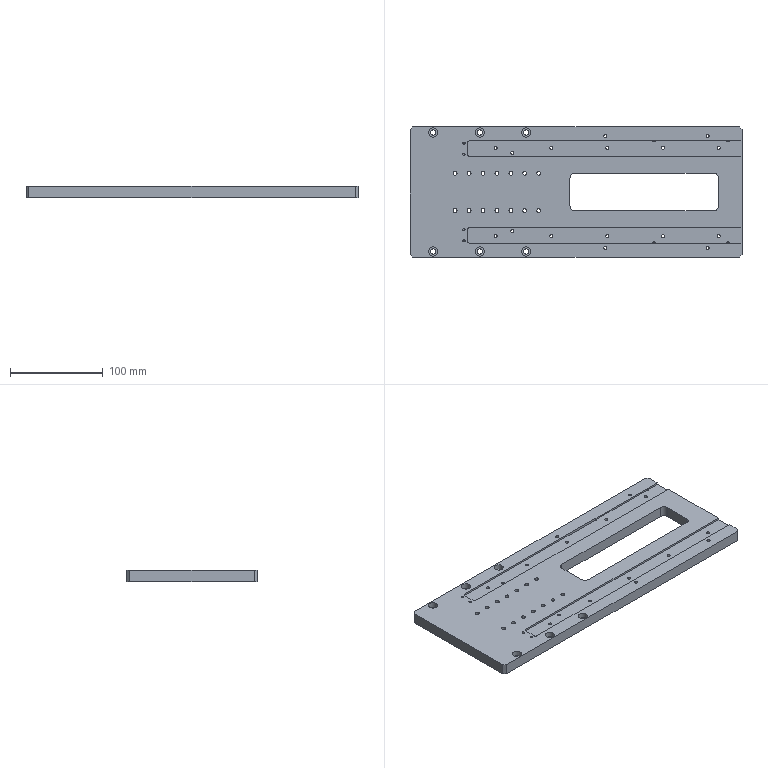NC program | NX | posted with a generic post | part box 357 x 140 x 12 mm
Whole program:
N10 G17 G21 G94 G90
(DRILLING , TOOL : D6A45)
N12 T01 M6
N14 G54
N16 G17 G0 G90 X153.5 Y-47.5 B0. C0. S9500 M3
N18 G43 Z30. H1
N20 G94 G81 G98 Z-1. F250. R3.
N22 X141.5 Y-60.
N24 X93.5 Y-47.5
N26 X33.5
N28 X31.5 Y-60.
N30 X-26.5 Y-47.5
N32 X-53.5 Y-64.
N34 X-68.5 Y-42.
N36 X-86.5 Y-47.5
N38 X-103.5 Y-64.
N40 X-120.5 Y-52.5
N42 X-153.5 Y-64.
N44 X-120.5 Y-40.5
N46 X-130. Y-20.
N48 X-115.
N50 X-100.
N52 X-85.
N54 X-70.
N56 X-55.
N58 X-40.
N60 Y20.
N62 X-55.
N64 X-70.
N66 X-85.
N68 X-100.
N70 X-115.
N72 X-130.
N74 X-120.5 Y40.5
N76 X-153.5 Y64.
N78 X-120.5 Y52.5
N80 X-103.5 Y64.
N82 X-86.5 Y47.5
N84 X-68.5 Y42.
N86 X-53.5 Y64.
N88 X-26.5 Y47.5
N90 X31.5 Y60.
N92 X33.5 Y47.5
N94 X93.5
N96 X141.5 Y60.
N98 X153.5 Y47.5
N100 G80
N102 G0 X153.5 Y47.5 Z30.
N104 M5
(DRILLING_COPY_COPY_COPY , TOOL : 2.5ZT)
N106 T02 M6
N108 G54
N110 G17 G0 G90 X-120.5 Y52.5 B0. C0. S2000 M3
N112 G43 Z30. H2
N114 G94 G83 G98 Z-8.101 F100. Q2. R3.
N116 Y40.5
N118 Y-40.5
N120 Y-52.5
N122 G80
N124 G0 X-120.5 Y-52.5 Z30.
N126 M5
(DRILLING_COPY_COPY , TOOL : 5.5ZT)
N128 T09 M6
N130 G54
N132 G17 G0 G90 X-153.5 Y-64. B0. C0. S2000 M3
N134 G43 Z30. H9
N136 G94 G83 G98 Z-14.152 F300. Q2. R3.
N138 X-103.5
N140 X-53.5
N142 Y64.
N144 X-103.5
N146 X-153.5
N148 G80
N150 G0 X-153.5 Y64. Z30.
N152 M5
(DRILLING_COPY_COPY_COPY_COPY , TOOL : 4.2ZT)
N154 T04 M6
N156 G54
N158 G17 G0 G90 X-40. Y20. B0. C0. S2000 M3
N160 G43 Z30. H4
N162 G94 G83 G98 Z-13.762 F300. Q2. R3.
N164 X-55.
N166 X-70.
N168 X-85.
N170 X-100.
N172 X-115.
N174 X-130.
N176 Y-20.
N178 X-115.
N180 X-100.
N182 X-85.
N184 X-70.
N186 X-55.
N188 X-40.
N190 G80
N192 G0 X-40. Y-20. Z30.
N194 M5
(DRILLING_COPY_COPY_COPY_1 , TOOL : 3.3ZT)
N196 T03 M6
N198 G54
N200 G17 G0 G90 X-86.5 Y-47.5 B0. C0. S2026 M3
N202 G43 Z30. H3
N204 G94 G83 G98 Z-13.491 F200. Q2. R3.
N206 X-68.5 Y-42.
N208 X-26.5 Y-47.5
N210 X33.5
N212 X93.5
N214 X153.5
N216 Y47.5
N218 X93.5
N220 X33.5
N222 X-26.5
N224 X-68.5 Y42.
N226 X-86.5 Y47.5
N228 G80
N230 G0 X-86.5 Y47.5 Z30.
N232 M5
(ZLEVEL_PROFILE , TOOL : D10)
N234 T15 M6
N236 G54
N238 G17 G0 G90 X175.718 Y79.678 B0. C0. S9500 M3
N240 G43 Z30. H15
N242 Z0.5
N244 G94 G1 Z-1. F1000.
N246 X175.3 Y78.117
N248 G3 X175.558 Y77.151 R1.
N250 G1 X178.707 Y74.002 F3000.
N252 X179.106 Y73.606
N254 X182.106 Y70.606
N256 G2 X183.6 Y67. R5.1
N258 G1 Y-65.997
N260 X183.537 Y-66.201
N262 G2 X182.106 Y-70.606 R5.1
N264 G1 X180.619 Y-72.094
N266 X180.58 Y-72.128
N268 X175.558 Y-77.151
N270 G3 X175.3 Y-78.117 R1.
N272 G1 X175.72 Y-79.686
N274 Z0.5
N276 G0 Z-0.5
N278 G1 Z-2. F1000.
N280 X175.3 Y-78.117
N282 G2 X175.558 Y-77.151 R1.
N284 G1 X180.58 Y-72.128 F3000.
N286 X182.106 Y-70.606
N288 G3 X183.537 Y-66.201 R5.1
N290 G1 X183.6 Y-65.997
N292 Y67.
N294 G3 X182.106 Y70.606 R5.1
N296 G1 X179.106 Y73.606
N298 X178.707 Y74.002
N300 X175.558 Y77.151
N302 G2 X175.3 Y78.117 R1.
N304 G1 X175.718 Y79.678
N306 Z-0.5
N308 G0 Z-1.5
N310 G1 Z-3. F1000.
N312 X175.3 Y78.117
N314 G3 X175.558 Y77.151 R1.
N316 G1 X178.707 Y74.002 F3000.
N318 X179.106 Y73.606
N320 X182.106 Y70.606
N322 G2 X183.6 Y67. R5.1
N324 G1 Y-65.997
N326 X183.537 Y-66.201
N328 G2 X182.106 Y-70.606 R5.1
N330 G1 X180.581 Y-72.128
N332 X175.558 Y-77.151
N334 G3 X175.3 Y-78.117 R1.
N336 G1 X175.72 Y-79.686
N338 Z-1.5
N340 G0 Z-2.5
N342 G1 Z-4. F1000.
N344 X175.3 Y-78.117
N346 G2 X175.559 Y-77.152 R1.
N348 G1 X180.619 Y-72.094 F3000.
N350 X182.106 Y-70.606
N352 G3 X183.537 Y-66.201 R5.1
N354 G1 X183.6 Y-65.997
N356 Y67.
N358 G3 X182.106 Y70.606 R5.1
N360 G1 X179.106 Y73.606
N362 X178.707 Y74.002
N364 X175.559 Y77.152
N366 G2 X175.3 Y78.117 R1.
N368 G1 X175.718 Y79.678
N370 Z-2.5
N372 G0 Z-3.5
N374 G1 Z-5. F1000.
N376 X175.3 Y78.118
N378 G3 X175.559 Y77.152 R1.
N380 G1 X178.707 Y74.002 F3000.
N382 X179.106 Y73.606
N384 X182.106 Y70.606
N386 G2 X183.6 Y67. R5.1
N388 G1 Y-65.997
N390 X183.537 Y-66.201
N392 G2 X182.106 Y-70.606 R5.1
N394 G1 X180.581 Y-72.128
N396 X175.559 Y-77.152
N398 G3 X175.3 Y-78.118 R1.
N400 G1 X175.721 Y-79.687
N402 Z-3.5
N404 G0 Z-4.5
N406 G1 Z-6. F1000.
N408 X175.3 Y-78.118
N410 G2 X175.559 Y-77.152 R1.
N412 G1 X180.619 Y-72.094 F3000.
N414 X182.106 Y-70.606
N416 G3 X183.537 Y-66.201 R5.1
N418 G1 X183.6 Y-65.997
N420 Y67.
N422 G3 X182.106 Y70.606 R5.1
N424 G1 X179.106 Y73.606
N426 X175.559 Y77.152
N428 G2 X175.3 Y78.118 R1.
N430 G1 X175.718 Y79.679
N432 Z-4.5
N434 G0 Z-5.5
N436 G1 Z-7. F1000.
N438 X175.3 Y78.118
N440 G3 X175.559 Y77.152 R1.
N442 G1 X179.106 Y73.606 F3000.
N444 X182.106 Y70.606
N446 G2 X183.6 Y67. R5.1
N448 G1 Y-65.997
N450 X183.537 Y-66.201
N452 G2 X182.106 Y-70.606 R5.1
N454 G1 X180.581 Y-72.128
N456 X175.559 Y-77.152
N458 G3 X175.3 Y-78.118 R1.
N460 G1 X175.721 Y-79.687
N462 Z-5.5
N464 G0 Z-6.5
N466 G1 Z-8. F1000.
N468 X175.3 Y-78.118
N470 G2 X175.559 Y-77.152 R1.
N472 G1 X180.619 Y-72.094 F3000.
N474 X182.106 Y-70.606
N476 G3 X183.537 Y-66.201 R5.1
N478 G1 X183.6 Y-65.997
N480 Y67.
N482 G3 X182.106 Y70.606 R5.1
N484 G1 X179.106 Y73.606
N486 X175.559 Y77.152
N488 G2 X175.3 Y78.118 R1.
N490 G1 X175.718 Y79.679
N492 Z-6.5
N494 G0 Z-7.5
N496 G1 Z-9. F1000.
N498 X175.3 Y78.118
N500 G3 X175.559 Y77.152 R1.
N502 G1 X179.106 Y73.606 F3000.
N504 X182.106 Y70.606
N506 G2 X183.6 Y67. R5.1
N508 G1 Y-65.997
N510 X183.537 Y-66.201
N512 G2 X182.106 Y-70.606 R5.1
N514 G1 X180.619 Y-72.094
N516 X175.559 Y-77.152
N518 G3 X175.3 Y-78.118 R1.
N520 G1 X175.72 Y-79.687
N522 Z-7.5
N524 G0 Z-8.5
N526 G1 Z-10. F1000.
N528 X175.3 Y-78.118
N530 G2 X175.559 Y-77.152 R1.
N532 G1 X180.619 Y-72.094 F3000.
N534 X182.106 Y-70.606
N536 G3 X183.537 Y-66.201 R5.1
N538 G1 X183.6 Y-65.997
N540 Y67.
N542 G3 X182.106 Y70.606 R5.1
N544 G1 X179.106 Y73.606
N546 X175.559 Y77.152
N548 G2 X175.3 Y78.118 R1.
N550 G1 X175.718 Y79.679
N552 Z-8.5
N554 G0 Z-9.5
N556 G1 Z-11. F1000.
N558 X175.3 Y78.118
N560 G3 X175.559 Y77.152 R1.
N562 G1 X179.106 Y73.606 F3000.
N564 X182.106 Y70.606
N566 G2 X183.6 Y67. R5.1
N568 G1 Y-65.997
N570 X183.537 Y-66.201
N572 G2 X182.106 Y-70.606 R5.1
N574 G1 X180.619 Y-72.094
N576 X175.559 Y-77.152
N578 G3 X175.3 Y-78.118 R1.
N580 G1 X175.721 Y-79.687
N582 Z-9.5
N584 G0 Y-79.688 Z-10.5
N586 G1 Z-12. F1000.
N588 X175.3 Y-78.118
N590 G2 X175.559 Y-77.152 R1.
N592 G1 X180.619 Y-72.094 F3000.
N594 X182.106 Y-70.606
N596 G3 X183.537 Y-66.201 R5.1
N598 G1 X183.6 Y-65.997
N600 Y67.
N602 G3 X182.106 Y70.606 R5.1
N604 G1 X179.106 Y73.606
N606 X175.559 Y77.152
N608 G2 X175.3 Y78.118 R1.
N610 G1 X175.718 Y79.679
N612 Z-10.5
N614 G0 Z30.
N616 X-175.718 Y-79.678
N618 Z0.5
N620 G1 Z-1. F1000.
N622 X-175.3 Y-78.117
N624 G3 X-175.558 Y-77.151 R1.
N626 G1 X-180.58 Y-72.128 F3000.
N628 X-180.619 Y-72.094
N630 X-182.106 Y-70.606
N632 G2 X-183.569 Y-66.438 R5.1
N634 G1 X-183.596 Y-66.387
N636 Y-65.997
N638 X-183.6 Y-65.948
N640 Y67.
N642 G2 X-182.106 Y70.606 R5.1
N644 G1 X-179.106 Y73.606
N646 X-178.51 Y74.198
N648 X-175.558 Y77.151
N650 G3 X-175.3 Y78.117 R1.
N652 G1 X-175.72 Y79.686
N654 Z0.5
N656 G0 Z-0.5
N658 G1 Z-2. F1000.
N660 X-175.3 Y78.117
N662 G2 X-175.558 Y77.151 R1.
N664 G1 X-178.51 Y74.198 F3000.
N666 X-179.106 Y73.606
N668 X-182.106 Y70.606
N670 G3 X-183.6 Y67. R5.1
N672 G1 Y-65.948
N674 X-183.596 Y-65.997
N676 Y-66.387
N678 X-183.569 Y-66.438
N680 G3 X-182.106 Y-70.606 R5.1
N682 G1 X-180.58 Y-72.128
N684 X-175.558 Y-77.151
N686 G2 X-175.3 Y-78.117 R1.
N688 G1 X-175.718 Y-79.678
N690 Z-0.5
N692 G0 Z-1.5
N694 G1 Z-3. F1000.
N696 X-175.3 Y-78.117
N698 G3 X-175.558 Y-77.151 R1.
N700 G1 X-180.619 Y-72.094 F3000.
N702 X-182.106 Y-70.606
N704 G2 X-183.569 Y-66.438 R5.1
N706 G1 X-183.596 Y-66.387
N708 Y-65.997
N710 X-183.6 Y-65.948
N712 Y67.
N714 G2 X-182.106 Y70.606 R5.1
N716 G1 X-179.106 Y73.606
N718 X-178.51 Y74.198
N720 X-175.558 Y77.151
N722 G3 X-175.3 Y78.117 R1.
N724 G1 X-175.721 Y79.686
N726 Z-1.5
N728 G0 Z-2.5
N730 G1 Z-4. F1000.
N732 X-175.3 Y78.117
N734 G2 X-175.559 Y77.152 R1.
N736 G1 X-178.511 Y74.198 F3000.
N738 X-179.106 Y73.606
N740 X-182.106 Y70.606
N742 G3 X-183.6 Y67. R5.1
N744 G1 Y-65.948
N746 X-183.596 Y-65.997
N748 Y-66.387
N750 X-183.569 Y-66.438
N752 G3 X-182.106 Y-70.606 R5.1
N754 G1 X-180.581 Y-72.128
N756 X-175.559 Y-77.152
N758 G2 X-175.3 Y-78.117 R1.
N760 G1 X-175.718 Y-79.678
N762 Z-2.5
N764 G0 Z-3.5
N766 G1 Z-5. F1000.
N768 X-175.3 Y-78.118
N770 G3 X-175.559 Y-77.152 R1.
N772 G1 X-180.619 Y-72.094 F3000.
N774 X-182.106 Y-70.606
N776 G2 X-183.569 Y-66.438 R5.1
N778 G1 X-183.596 Y-66.387
N780 Y-65.997
N782 X-183.6 Y-65.948
N784 Y67.
N786 G2 X-182.106 Y70.606 R5.1
N788 G1 X-179.106 Y73.606
N790 X-178.511 Y74.199
N792 X-175.559 Y77.152
N794 G3 X-175.3 Y78.118 R1.
N796 G1 X-175.721 Y79.686
N798 Z-3.5
N800 G0 X-175.72 Y79.687 Z-4.5
N802 G1 Z-6. F1000.
N804 X-175.3 Y78.118
N806 G2 X-175.559 Y77.152 R1.
N808 G1 X-179.106 Y73.606 F3000.
N810 X-182.106 Y70.606
N812 G3 X-183.6 Y67. R5.1
N814 G1 Y-65.948
N816 X-183.596 Y-65.997
N818 Y-66.387
N820 X-183.569 Y-66.438
N822 G3 X-182.106 Y-70.606 R5.1
N824 G1 X-180.581 Y-72.128
N826 X-175.559 Y-77.152
N828 G2 X-175.3 Y-78.118 R1.
N830 G1 X-175.718 Y-79.678
N832 Z-4.5
N834 G0 Z-5.5
N836 G1 Z-7. F1000.
N838 X-175.3 Y-78.118
N840 G3 X-175.559 Y-77.152 R1.
N842 G1 X-180.619 Y-72.094 F3000.
N844 X-182.106 Y-70.606
N846 G2 X-183.569 Y-66.438 R5.1
N848 G1 X-183.596 Y-66.387
N850 Y-65.997
N852 X-183.6 Y-65.948
N854 Y67.
N856 G2 X-182.106 Y70.606 R5.1
N858 G1 X-179.106 Y73.606
N860 X-175.559 Y77.152
N862 G3 X-175.3 Y78.118 R1.
N864 G1 X-175.72 Y79.687
N866 Z-5.5
N868 G0 Z-6.5
N870 G1 Z-8. F1000.
N872 X-175.3 Y78.118
N874 G2 X-175.559 Y77.152 R1.
N876 G1 X-179.106 Y73.606 F3000.
N878 X-182.106 Y70.606
N880 G3 X-183.6 Y67. R5.1
N882 G1 Y-65.948
N884 X-183.596 Y-65.997
N886 Y-66.387
N888 X-183.569 Y-66.438
N890 G3 X-182.106 Y-70.606 R5.1
N892 G1 X-180.581 Y-72.129
N894 X-175.559 Y-77.152
N896 G2 X-175.3 Y-78.118 R1.
N898 G1 X-175.719 Y-79.678
N900 Z-6.5
N902 G0 X-175.718 Y-79.679 Z-7.5
N904 G1 Z-9. F1000.
N906 X-175.3 Y-78.118
N908 G3 X-175.559 Y-77.152 R1.
N910 G1 X-180.619 Y-72.094 F3000.
N912 X-182.106 Y-70.606
N914 G2 X-183.569 Y-66.438 R5.1
N916 G1 X-183.596 Y-66.387
N918 Y-65.997
N920 X-183.6 Y-65.948
N922 Y67.
N924 G2 X-182.106 Y70.606 R5.1
N926 G1 X-179.106 Y73.606
N928 X-175.559 Y77.152
N930 G3 X-175.3 Y78.118 R1.
N932 G1 X-175.72 Y79.687
N934 Z-7.5
N936 G0 Y79.688 Z-8.5
N938 G1 Z-10. F1000.
N940 X-175.3 Y78.118
N942 G2 X-175.559 Y77.152 R1.
N944 G1 X-179.106 Y73.606 F3000.
N946 X-182.106 Y70.606
N948 G3 X-183.6 Y67. R5.1
N950 G1 Y-65.948
N952 X-183.596 Y-65.997
N954 Y-66.387
N956 X-183.569 Y-66.438
N958 G3 X-182.106 Y-70.606 R5.1
N960 G1 X-180.619 Y-72.094
N962 X-175.559 Y-77.152
N964 G2 X-175.3 Y-78.118 R1.
N966 G1 X-175.718 Y-79.679
N968 Z-8.5
N970 G0 Z-9.5
N972 G1 Z-11. F1000.
N974 X-175.3 Y-78.118
N976 G3 X-175.559 Y-77.152 R1.
N978 G1 X-180.619 Y-72.094 F3000.
N980 X-182.106 Y-70.606
N982 G2 X-183.569 Y-66.438 R5.1
N984 G1 X-183.596 Y-66.387
N986 Y-65.997
N988 X-183.6 Y-65.948
N990 Y67.
N992 G2 X-182.106 Y70.606 R5.1
N994 G1 X-179.106 Y73.606
N996 X-175.559 Y77.152
N998 G3 X-175.3 Y78.118 R1.
N1000 G1 X-175.72 Y79.688
N1002 Z-9.5
N1004 G0 X-175.721 Z-10.5
N1006 G1 Z-12. F1000.
N1008 X-175.3 Y78.118
N1010 G2 X-175.559 Y77.152 R1.
N1012 G1 X-179.106 Y73.606 F3000.
N1014 X-182.106 Y70.606
N1016 G3 X-183.6 Y67. R5.1
N1018 G1 Y-65.948
N1020 X-183.596 Y-65.997
N1022 Y-66.387
N1024 X-183.569 Y-66.438
N1026 G3 X-182.106 Y-70.606 R5.1
N1028 G1 X-180.619 Y-72.094
N1030 X-175.559 Y-77.152
N1032 G2 X-175.3 Y-78.118 R1.
N1034 G1 X-175.718 Y-79.679
N1036 Z-10.5
N1038 G0 Z30.
(PLANAR_MILL , TOOL : D10)
N1040 X25.797 Y-0.4
N1042 Z1.5
N1044 G1 X73.5 Z-1. F1000.
N1046 X133.9 F3000.
N1048 Y0.4
N1050 X13.1
N1052 Y-0.4
N1054 X73.5
N1056 Y-4.9
N1058 X138.4
N1060 Y4.9
N1062 X8.6
N1064 Y-4.9
N1066 X73.5
N1068 Y-9.9
N1070 X143.4
N1072 Y9.9
N1074 X3.6
N1076 Y-9.9
N1078 X73.5
N1080 Y-14.9
N1082 X148.4
N1084 Y14.9
N1086 X-1.4
N1088 Y-14.9
N1090 X73.5
N1092 Z0.5
N1094 G0 X25.797 Y-0.4
N1096 G1 X73.5 Z-2. F1000.
N1098 X133.9 F3000.
N1100 Y0.4
N1102 X13.1
N1104 Y-0.4
N1106 X73.5
N1108 Y-4.9
N1110 X138.4
N1112 Y4.9
N1114 X8.6
N1116 Y-4.9
N1118 X73.5
N1120 Y-9.9
N1122 X143.4
N1124 Y9.9
N1126 X3.6
N1128 Y-9.9
N1130 X73.5
N1132 Y-14.9
N1134 X148.4
N1136 Y14.9
N1138 X-1.4
N1140 Y-14.9
N1142 X73.5
N1144 Z-0.5
N1146 G0 X25.797 Y-0.4
N1148 G1 X73.5 Z-3. F1000.
N1150 X133.9 F3000.
N1152 Y0.4
N1154 X13.1
N1156 Y-0.4
N1158 X73.5
N1160 Y-4.9
N1162 X138.4
N1164 Y4.9
N1166 X8.6
N1168 Y-4.9
N1170 X73.5
N1172 Y-9.9
N1174 X143.4
N1176 Y9.9
N1178 X3.6
N1180 Y-9.9
N1182 X73.5
N1184 Y-14.9
N1186 X148.4
N1188 Y14.9
N1190 X-1.4
N1192 Y-14.9
N1194 X73.5
N1196 Z-1.5
N1198 G0 X25.797 Y-0.4
N1200 G1 X73.5 Z-4. F1000.
N1202 X133.9 F3000.
N1204 Y0.4
N1206 X13.1
N1208 Y-0.4
N1210 X73.5
N1212 Y-4.9
N1214 X138.4
N1216 Y4.9
N1218 X8.6
N1220 Y-4.9
N1222 X73.5
N1224 Y-9.9
N1226 X143.4
N1228 Y9.9
N1230 X3.6
N1232 Y-9.9
N1234 X73.5
N1236 Y-14.9
N1238 X148.4
N1240 Y14.9
N1242 X-1.4
N1244 Y-14.9
N1246 X73.5
N1248 Z-2.5
N1250 G0 X25.797 Y-0.4
N1252 G1 X73.5 Z-5. F1000.
N1254 X133.9 F3000.
N1256 Y0.4
N1258 X13.1
N1260 Y-0.4
N1262 X73.5
N1264 Y-4.9
N1266 X138.4
N1268 Y4.9
N1270 X8.6
N1272 Y-4.9
N1274 X73.5
N1276 Y-9.9
N1278 X143.4
N1280 Y9.9
N1282 X3.6
N1284 Y-9.9
N1286 X73.5
N1288 Y-14.9
N1290 X148.4
N1292 Y14.9
N1294 X-1.4
N1296 Y-14.9
N1298 X73.5
N1300 Z-3.5
N1302 G0 X25.797 Y-0.4
N1304 G1 X73.5 Z-6. F1000.
N1306 X133.9 F3000.
N1308 Y0.4
N1310 X13.1
N1312 Y-0.4
N1314 X73.5
N1316 Y-4.9
N1318 X138.4
N1320 Y4.9
N1322 X8.6
N1324 Y-4.9
N1326 X73.5
N1328 Y-9.9
N1330 X143.4
N1332 Y9.9
N1334 X3.6
N1336 Y-9.9
N1338 X73.5
N1340 Y-14.9
N1342 X148.4
N1344 Y14.9
N1346 X-1.4
N1348 Y-14.9
N1350 X73.5
N1352 Z-4.5
N1354 G0 X25.797 Y-0.4
N1356 G1 X73.5 Z-7. F1000.
N1358 X133.9 F3000.
N1360 Y0.4
N1362 X13.1
N1364 Y-0.4
N1366 X73.5
N1368 Y-4.9
N1370 X138.4
N1372 Y4.9
N1374 X8.6
N1376 Y-4.9
N1378 X73.5
N1380 Y-9.9
N1382 X143.4
N1384 Y9.9
N1386 X3.6
N1388 Y-9.9
N1390 X73.5
N1392 Y-14.9
N1394 X148.4
N1396 Y14.9
N1398 X-1.4
N1400 Y-14.9
N1402 X73.5
N1404 Z-5.5
N1406 G0 X25.797 Y-0.4
N1408 G1 X73.5 Z-8. F1000.
N1410 X133.9 F3000.
N1412 Y0.4
N1414 X13.1
N1416 Y-0.4
N1418 X73.5
N1420 Y-4.9
N1422 X138.4
N1424 Y4.9
N1426 X8.6
N1428 Y-4.9
N1430 X73.5
N1432 Y-9.9
N1434 X143.4
N1436 Y9.9
N1438 X3.6
N1440 Y-9.9
N1442 X73.5
N1444 Y-14.9
N1446 X148.4
N1448 Y14.9
N1450 X-1.4
N1452 Y-14.9
N1454 X73.5
N1456 Z-6.5
N1458 G0 X25.797 Y-0.4
N1460 G1 X73.5 Z-9. F1000.
N1462 X133.9 F3000.
N1464 Y0.4
N1466 X13.1
N1468 Y-0.4
N1470 X73.5
N1472 Y-4.9
N1474 X138.4
N1476 Y4.9
N1478 X8.6
N1480 Y-4.9
N1482 X73.5
N1484 Y-9.9
N1486 X143.4
N1488 Y9.9
N1490 X3.6
N1492 Y-9.9
N1494 X73.5
N1496 Y-14.9
N1498 X148.4
N1500 Y14.9
N1502 X-1.4
N1504 Y-14.9
N1506 X73.5
N1508 Z-7.5
N1510 G0 X25.797 Y-0.4
N1512 G1 X73.5 Z-10. F1000.
N1514 X133.9 F3000.
N1516 Y0.4
N1518 X13.1
N1520 Y-0.4
N1522 X73.5
N1524 Y-4.9
N1526 X138.4
N1528 Y4.9
N1530 X8.6
N1532 Y-4.9
N1534 X73.5
N1536 Y-9.9
N1538 X143.4
N1540 Y9.9
N1542 X3.6
N1544 Y-9.9
N1546 X73.5
N1548 Y-14.9
N1550 X148.4
N1552 Y14.9
N1554 X-1.4
N1556 Y-14.9
N1558 X73.5
N1560 Z-8.5
N1562 G0 X25.797 Y-0.4
N1564 G1 X73.5 Z-11. F1000.
N1566 X133.9 F3000.
N1568 Y0.4
N1570 X13.1
N1572 Y-0.4
N1574 X73.5
N1576 Y-4.9
N1578 X138.4
N1580 Y4.9
N1582 X8.6
N1584 Y-4.9
N1586 X73.5
N1588 Y-9.9
N1590 X143.4
N1592 Y9.9
N1594 X3.6
N1596 Y-9.9
N1598 X73.5
N1600 Y-14.9
N1602 X148.4
N1604 Y14.9
N1606 X-1.4
N1608 Y-14.9
N1610 X73.5
N1612 Z-9.5
N1614 G0 X25.797 Y-0.4
N1616 G1 X73.5 Z-12. F1000.
N1618 X133.9 F3000.
N1620 Y0.4
N1622 X13.1
N1624 Y-0.4
N1626 X73.5
N1628 Y-4.9
N1630 X138.4
N1632 Y4.9
N1634 X8.6
N1636 Y-4.9
N1638 X73.5
N1640 Y-9.9
N1642 X143.4
N1644 Y9.9
N1646 X3.6
N1648 Y-9.9
N1650 X73.5
N1652 Y-14.9
N1654 X148.4
N1656 Y14.9
N1658 X-1.4
N1660 Y-14.9
N1662 X73.5
N1664 Z-10.5
N1666 G0 Z30.
(FLOOR_WALL , TOOL : D10)
N1668 X185.1 Y50.599
N1670 Z0.55
N1672 G1 Z-0.95 F2500.
N1674 X178.75 Y46.933
N1676 G3 X178.5 Y46.5 R0.5
N1678 G1 Y43.1
N1680 X-111.4
N1682 Y49.9
N1684 X178.5
N1686 Y46.5
N1688 G3 X178.75 Y46.067 R0.5
N1690 G1 X185.1 Y42.401
N1692 Z0.55
N1694 G0 Y50.599 Z-0.4
N1696 G1 Z-1.9
N1698 X178.75 Y46.933
N1700 G3 X178.5 Y46.5 R0.5
N1702 G1 Y43.1
N1704 X-111.4
N1706 Y49.9
N1708 X178.5
N1710 Y46.5
N1712 G3 X179. Y45.634 R1.
N1714 G1 X185.1 Y42.112
N1716 Z-0.4
N1718 G0 Z30.
N1720 Y-42.401
N1722 Z0.55
N1724 G1 Z-0.95
N1726 X178.75 Y-46.067
N1728 G3 X178.5 Y-46.5 R0.5
N1730 G1 Y-49.9
N1732 X-111.4
N1734 Y-43.1
N1736 X178.5
N1738 Y-46.5
N1740 G3 X178.75 Y-46.933 R0.5
N1742 G1 X185.1 Y-50.599
N1744 Z0.55
N1746 G0 Y-42.401 Z-0.4
N1748 G1 Z-1.9
N1750 X178.75 Y-46.067
N1752 G3 X178.5 Y-46.5 R0.5
N1754 G1 Y-49.9
N1756 X-111.4
N1758 Y-43.1
N1760 X178.5
N1762 Y-46.5
N1764 G3 X178.75 Y-46.933 R0.5
N1766 G1 X185.1 Y-50.599
N1768 Z-0.4
N1770 G0 Z30.
N1772 M5
(FLOOR_WALL_1 , TOOL : D10JING)
N1774 T14 M6
N1776 G54
N1778 G17 G0 G90 X185. Y-68.955 B0. C0. S9500 M3
N1780 G43 Z30. H14
N1782 Z-10.5
N1784 G94 G1 Z-12. F1250.
N1786 X184.466 Y-68.812
N1788 G3 X183.5 Y-69.071 R1.
N1790 G1 X180.085 Y-72.486
N1792 G3 X179.826 Y-73.452 R1.
N1794 G1 X180.125 Y-74.567
N1796 Z-10.5
N1798 G0 Z30.
N1800 X177.455 Y76.5
N1802 Z-10.5
N1804 G1 Z-12.
N1806 X177.312 Y75.966
N1808 G3 X177.571 Y75. R1.
N1810 G1 X183.5 Y69.071
N1812 G3 X184.466 Y68.812 R1.
N1814 G1 X185. Y68.955
N1816 Z-10.5
N1818 G0 Z30.
N1820 X74.943 Y13.5
N1822 Z-10.5
N1824 G1 Z-12.
N1826 X74.366 Y14.5
N1828 G3 X73.5 Y15. R1.
N1830 G1 X-1.5
N1832 Y-15.
N1834 X148.5
N1836 Y15.
N1838 X73.5
N1840 G3 X72.634 Y14.5 R1.
N1842 G1 X72.057 Y13.5
N1844 Z-10.5
N1846 G0 Z30.
N1848 X-177.455 Y-76.5
N1850 Z-10.5
N1852 G1 Z-12.
N1854 X-177.312 Y-75.966
N1856 G3 X-177.571 Y-75. R1.
N1858 G1 X-183.5 Y-69.071
N1860 Y69.071
N1862 X-177.571 Y75.
N1864 G3 X-177.312 Y75.966 R1.
N1866 G1 X-177.455 Y76.5
N1868 Z-10.5
N1870 G0 Z30.
N1872 M5
(ZLEVEL_PROFILE_COPY , TOOL : D4)
N1874 T11 M6
N1876 G54
N1878 G17 G0 G90 X-110.91 Y52.2 B0. C0. S9500 M3
N1880 G43 Z30. H11
N1882 Z-0.4
N1884 G94 G1 X-111.257 Y52.8 F1000.
N1886 G3 X-111.603 Y53. R0.4
N1888 G1 X-114.5 F1500.
N1890 Y50.103
N1892 G3 X-114.3 Y49.757 R0.4
N1894 G1 X-113.7 Y49.41
N1896 G0 X-110.91 Y52.2 Z-0.8
N1898 G1 X-111.257 Y52.8 F1000.
N1900 G3 X-111.603 Y53. R0.4
N1902 G1 X-114.5 F1500.
N1904 Y50.103
N1906 G3 X-114.3 Y49.757 R0.4
N1908 G1 X-113.7 Y49.41
N1910 G0 X-110.91 Y52.2 Z-1.2
N1912 G1 X-111.257 Y52.8 F1000.
N1914 G3 X-111.603 Y53. R0.4
N1916 G1 X-114.5 F1500.
N1918 Y50.103
N1920 G3 X-114.3 Y49.757 R0.4
N1922 G1 X-113.7 Y49.41
N1924 G0 X-110.91 Y52.2 Z-1.6
N1926 G1 X-111.257 Y52.8 F1000.
N1928 G3 X-111.603 Y53. R0.4
N1930 G1 X-114.5 F1500.
N1932 Y50.103
N1934 G3 X-114.3 Y49.757 R0.4
N1936 G1 X-113.7 Y49.41
N1938 G0 X-110.91 Y52.2 Z-2.
N1940 G1 X-111.257 Y52.8 F1000.
N1942 G3 X-111.603 Y53. R0.4
N1944 G1 X-114.5 F1500.
N1946 Y50.103
N1948 G3 X-114.3 Y49.757 R0.4
N1950 G1 X-113.7 Y49.41
N1952 G0 Z30.
N1954 Y43.59
N1956 Z-0.4
N1958 G1 X-114.3 Y43.243 F1000.
N1960 G3 X-114.5 Y42.897 R0.4
N1962 G1 Y40.481 F1500.
N1964 X-114.501 Y40.001
N1966 X-114.411 Y40.
N1968 X-111.603
N1970 G3 X-111.257 Y40.2 R0.4
N1972 G1 X-110.91 Y40.8
N1974 G0 X-113.7 Y43.59 Z-0.8
N1976 G1 X-114.3 Y43.243 F1000.
N1978 G3 X-114.5 Y42.897 R0.4
N1980 G1 Y40.481 F1500.
N1982 Y40.001
N1984 X-114.411 Y40.
N1986 X-111.603
N1988 G3 X-111.257 Y40.2 R0.4
N1990 G1 X-110.91 Y40.8
N1992 G0 X-113.7 Y43.59 Z-1.2
N1994 G1 X-114.3 Y43.243 F1000.
N1996 G3 X-114.5 Y42.897 R0.4
N1998 G1 Y40.002 F1500.
N2000 X-114.411 Y40.
N2002 X-111.603
N2004 G3 X-111.257 Y40.2 R0.4
N2006 G1 X-110.91 Y40.8
N2008 G0 X-113.7 Y43.59 Z-1.6
N2010 G1 X-114.3 Y43.243 F1000.
N2012 G3 X-114.5 Y42.897 R0.4
N2014 G1 Y40.002 F1500.
N2016 X-114.411 Y40.
N2018 X-111.603
N2020 G3 X-111.257 Y40.2 R0.4
N2022 G1 X-110.91 Y40.8
N2024 G0 X-113.7 Y43.59 Z-2.
N2026 G1 X-114.3 Y43.243 F1000.
N2028 G3 X-114.5 Y42.897 R0.4
N2030 G1 Y40.003 F1500.
N2032 X-114.411 Y40.
N2034 X-111.603
N2036 G3 X-111.257 Y40.2 R0.4
N2038 G1 X-110.91 Y40.8
N2040 G0 Z30.
N2042 Y-40.8
N2044 Z-0.4
N2046 G1 X-111.257 Y-40.2 F1000.
N2048 G3 X-111.603 Y-40. R0.4
N2050 G1 X-114.411 F1500.
N2052 X-114.5
N2054 Y-42.897
N2056 G3 X-114.3 Y-43.243 R0.4
N2058 G1 X-113.7 Y-43.59
N2060 G0 X-110.91 Y-40.8 Z-0.8
N2062 G1 X-111.257 Y-40.2 F1000.
N2064 G3 X-111.603 Y-40. R0.4
N2066 G1 X-114.411 F1500.
N2068 X-114.5
N2070 Y-42.897
N2072 G3 X-114.3 Y-43.243 R0.4
N2074 G1 X-113.7 Y-43.59
N2076 G0 X-110.91 Y-40.8 Z-1.2
N2078 G1 X-111.257 Y-40.2 F1000.
N2080 G3 X-111.603 Y-40. R0.4
N2082 G1 X-114.5 F1500.
N2084 Y-42.897
N2086 G3 X-114.3 Y-43.243 R0.4
N2088 G1 X-113.7 Y-43.59
N2090 G0 X-110.91 Y-40.8 Z-1.6
N2092 G1 X-111.257 Y-40.2 F1000.
N2094 G3 X-111.603 Y-40. R0.4
N2096 G1 X-114.5 F1500.
N2098 Y-42.897
N2100 G3 X-114.3 Y-43.243 R0.4
N2102 G1 X-113.7 Y-43.59
N2104 G0 X-110.91 Y-40.8 Z-2.
N2106 G1 X-111.257 Y-40.2 F1000.
N2108 G3 X-111.603 Y-40. R0.4
N2110 G1 X-114.5 F1500.
N2112 Y-42.897
N2114 G3 X-114.3 Y-43.243 R0.4
N2116 G1 X-113.7 Y-43.59
N2118 G0 Z30.
N2120 Y-49.41
N2122 Z-0.4
N2124 G1 X-114.3 Y-49.757 F1000.
N2126 G3 X-114.5 Y-50.103 R0.4
N2128 G1 Y-53. F1500.
N2130 X-111.603
N2132 G3 X-111.257 Y-52.8 R0.4
N2134 G1 X-110.91 Y-52.2
N2136 G0 X-113.7 Y-49.41 Z-0.8
N2138 G1 X-114.3 Y-49.757 F1000.
N2140 G3 X-114.5 Y-50.103 R0.4
N2142 G1 Y-53. F1500.
N2144 X-111.603
N2146 G3 X-111.257 Y-52.8 R0.4
N2148 G1 X-110.91 Y-52.2
N2150 G0 X-113.7 Y-49.41 Z-1.2
N2152 G1 X-114.3 Y-49.757 F1000.
N2154 G3 X-114.5 Y-50.103 R0.4
N2156 G1 Y-53. F1500.
N2158 X-111.603
N2160 G3 X-111.257 Y-52.8 R0.4
N2162 G1 X-110.91 Y-52.2
N2164 G0 X-113.7 Y-49.41 Z-1.6
N2166 G1 X-114.3 Y-49.757 F1000.
N2168 G3 X-114.5 Y-50.103 R0.4
N2170 G1 Y-53. F1500.
N2172 X-111.603
N2174 G3 X-111.257 Y-52.8 R0.4
N2176 G1 X-110.91 Y-52.2
N2178 G0 X-113.7 Y-49.41 Z-2.
N2180 G1 X-114.3 Y-49.757 F1000.
N2182 G3 X-114.5 Y-50.103 R0.4
N2184 G1 Y-53. F1500.
N2186 X-111.603
N2188 G3 X-111.257 Y-52.8 R0.4
N2190 G1 X-110.91 Y-52.2
N2192 G0 Z30.
(FLOOR_WALL_COPY , TOOL : D4)
N2194 X182. Y40.403
N2196 Z-0.5
N2198 G1 Z-2. F1350.
N2200 X180.154
N2202 G3 X180.5 Y40.203 R0.4
N2204 G1 X-114.3
N2206 Y42.003
N2208 X180.5
N2210 Y43.802
N2212 X-114.3
N2214 Y45.602
N2216 X180.5
N2218 Y47.401
N2220 X-114.3
N2222 Y49.201
N2224 X180.5
N2226 Y51.
N2228 X-114.3
N2230 Y52.8
N2232 X180.5
N2234 G2 X180.846 Y52.6 R0.4
N2236 G1 X182. Y50.602
N2238 Z-0.5
N2240 G0 Z3.
N2242 Y50.802
N2244 Z-0.5
N2246 G1 Z-2.
N2248 X180.846 Y52.8
N2250 G3 X180.5 Y53. R0.4
N2252 G1 X-114.5
N2254 Y40.
N2256 X180.5
N2258 G3 X180.846 Y40.2 R0.4
N2260 G1 X182. Y42.198
N2262 Z-0.5
N2264 G0 Z30.
N2266 Y-52.597
N2268 Z-0.5
N2270 G1 Z-2.
N2272 X180.154
N2274 G3 X180.5 Y-52.797 R0.4
N2276 G1 X-114.3
N2278 Y-50.997
N2280 X180.5
N2282 Y-49.198
N2284 X-114.3
N2286 Y-47.398
N2288 X180.5
N2290 Y-45.599
N2292 X-114.3
N2294 Y-43.799
N2296 X180.5
N2298 Y-42.
N2300 X-114.3
N2302 Y-40.2
N2304 X180.5
N2306 G2 X180.846 Y-40.4 R0.4
N2308 G1 X182. Y-42.398
N2310 Z-0.5
N2312 G0 Z3.
N2314 Y-42.198
N2316 Z-0.5
N2318 G1 Z-2.
N2320 X180.846 Y-40.2
N2322 G3 X180.5 Y-40. R0.4
N2324 G1 X-114.5
N2326 Y-53.
N2328 X180.5
N2330 G3 X180.846 Y-52.8 R0.4
N2332 G1 X182. Y-50.802
N2334 Z-0.5
N2336 G0 Z30.
(HOLE_MILLING , TOOL : D4)
N2338 X-153.5 Y64.
N2340 Z0.5
N2342 G3 X-152.763 Y63.263 R0.737 F1500.
N2344 X-152.025 Y64. R0.737
N2346 X-152.025 Y64. Z0.1 I-1.475 J0.
N2348 X-152.025 Y64. Z-0.3 I-1.475 J0.
N2350 X-152.025 Y64. Z-0.7 I-1.475 J0.
N2352 X-152.025 Y64. Z-1.1 I-1.475 J0.
N2354 X-152.025 Y64. Z-1.5 I-1.475 J0.
N2356 X-152.025 Y64. Z-1.9 I-1.475 J0.
N2358 X-152.025 Y64. Z-2.3 I-1.475 J0.
N2360 X-152.025 Y64. Z-2.7 I-1.475 J0.
N2362 X-152.025 Y64. Z-3.1 I-1.475 J0.
N2364 X-152.025 Y64. Z-3.5 I-1.475 J0.
N2366 X-152.025 Y64. Z-3.9 I-1.475 J0.
N2368 X-152.025 Y64. Z-4.3 I-1.475 J0.
N2370 X-152.025 Y64. Z-4.7 I-1.475 J0.
N2372 X-152.025 Y64. Z-5.1 I-1.475 J0.
N2374 X-152.025 Y64. Z-5.5 I-1.475 J0.
N2376 X-154.975 Y64. Z-5.7 I-1.475 J0.
N2378 X-153.5 Y62.525 R1.475
N2380 X-154.975 Y64. R-1.475
N2382 X-154.238 Y63.263 R0.737
N2384 X-153.5 Y64. R0.737
N2386 G0 Z0.5
N2388 G3 X-152.025 Y62.525 R1.475
N2390 X-150.55 Y64. R1.475
N2392 X-150.55 Y64. Z0.1 I-2.95 J0.
N2394 X-150.55 Y64. Z-0.3 I-2.95 J0.
N2396 X-150.55 Y64. Z-0.7 I-2.95 J0.
N2398 X-150.55 Y64. Z-1.1 I-2.95 J0.
N2400 X-150.55 Y64. Z-1.5 I-2.95 J0.
N2402 X-150.55 Y64. Z-1.9 I-2.95 J0.
N2404 X-150.55 Y64. Z-2.3 I-2.95 J0.
N2406 X-150.55 Y64. Z-2.7 I-2.95 J0.
N2408 X-150.55 Y64. Z-3.1 I-2.95 J0.
N2410 X-150.55 Y64. Z-3.5 I-2.95 J0.
N2412 X-150.55 Y64. Z-3.9 I-2.95 J0.
N2414 X-150.55 Y64. Z-4.3 I-2.95 J0.
N2416 X-150.55 Y64. Z-4.7 I-2.95 J0.
N2418 X-150.55 Y64. Z-5.1 I-2.95 J0.
N2420 X-150.55 Y64. Z-5.5 I-2.95 J0.
N2422 X-156.45 Y64. Z-5.7 I-2.95 J0.
N2424 X-153.5 Y61.05 R2.95
N2426 X-156.45 Y64. R-2.95
N2428 X-154.975 Y62.525 R1.475
N2430 X-153.5 Y64. R1.475
N2432 G0 Z30.
N2434 X-103.5
N2436 Z0.5
N2438 G3 X-102.763 Y63.263 R0.737
N2440 X-102.025 Y64. R0.737
N2442 X-102.025 Y64. Z0.1 I-1.475 J0.
N2444 X-102.025 Y64. Z-0.3 I-1.475 J0.
N2446 X-102.025 Y64. Z-0.7 I-1.475 J0.
N2448 X-102.025 Y64. Z-1.1 I-1.475 J0.
N2450 X-102.025 Y64. Z-1.5 I-1.475 J0.
N2452 X-102.025 Y64. Z-1.9 I-1.475 J0.
N2454 X-102.025 Y64. Z-2.3 I-1.475 J0.
N2456 X-102.025 Y64. Z-2.7 I-1.475 J0.
N2458 X-102.025 Y64. Z-3.1 I-1.475 J0.
N2460 X-102.025 Y64. Z-3.5 I-1.475 J0.
N2462 X-102.025 Y64. Z-3.9 I-1.475 J0.
N2464 X-102.025 Y64. Z-4.3 I-1.475 J0.
N2466 X-102.025 Y64. Z-4.7 I-1.475 J0.
N2468 X-102.025 Y64. Z-5.1 I-1.475 J0.
N2470 X-102.025 Y64. Z-5.5 I-1.475 J0.
N2472 X-104.975 Y64. Z-5.7 I-1.475 J0.
N2474 X-103.5 Y62.525 R1.475
N2476 X-104.975 Y64. R-1.475
N2478 X-104.238 Y63.263 R0.737
N2480 X-103.5 Y64. R0.737
N2482 G0 Z0.5
N2484 G3 X-102.025 Y62.525 R1.475
N2486 X-100.55 Y64. R1.475
N2488 X-100.55 Y64. Z0.1 I-2.95 J0.
N2490 X-100.55 Y64. Z-0.3 I-2.95 J0.
N2492 X-100.55 Y64. Z-0.7 I-2.95 J0.
N2494 X-100.55 Y64. Z-1.1 I-2.95 J0.
N2496 X-100.55 Y64. Z-1.5 I-2.95 J0.
N2498 X-100.55 Y64. Z-1.9 I-2.95 J0.
N2500 X-100.55 Y64. Z-2.3 I-2.95 J0.
N2502 X-100.55 Y64. Z-2.7 I-2.95 J0.
N2504 X-100.55 Y64. Z-3.1 I-2.95 J0.
N2506 X-100.55 Y64. Z-3.5 I-2.95 J0.
N2508 X-100.55 Y64. Z-3.9 I-2.95 J0.
N2510 X-100.55 Y64. Z-4.3 I-2.95 J0.
N2512 X-100.55 Y64. Z-4.7 I-2.95 J0.
N2514 X-100.55 Y64. Z-5.1 I-2.95 J0.
N2516 X-100.55 Y64. Z-5.5 I-2.95 J0.
N2518 X-106.45 Y64. Z-5.7 I-2.95 J0.
N2520 X-103.5 Y61.05 R2.95
N2522 X-106.45 Y64. R-2.95
N2524 X-104.975 Y62.525 R1.475
N2526 X-103.5 Y64. R1.475
N2528 G0 Z30.
N2530 X-53.5
N2532 Z0.5
N2534 G3 X-52.763 Y63.263 R0.738
N2536 X-52.025 Y64. R0.738
N2538 X-52.025 Y64. Z0.1 I-1.475 J0.
N2540 X-52.025 Y64. Z-0.3 I-1.475 J0.
N2542 X-52.025 Y64. Z-0.7 I-1.475 J0.
N2544 X-52.025 Y64. Z-1.1 I-1.475 J0.
N2546 X-52.025 Y64. Z-1.5 I-1.475 J0.
N2548 X-52.025 Y64. Z-1.9 I-1.475 J0.
N2550 X-52.025 Y64. Z-2.3 I-1.475 J0.
N2552 X-52.025 Y64. Z-2.7 I-1.475 J0.
N2554 X-52.025 Y64. Z-3.1 I-1.475 J0.
N2556 X-52.025 Y64. Z-3.5 I-1.475 J0.
N2558 X-52.025 Y64. Z-3.9 I-1.475 J0.
N2560 X-52.025 Y64. Z-4.3 I-1.475 J0.
N2562 X-52.025 Y64. Z-4.7 I-1.475 J0.
N2564 X-52.025 Y64. Z-5.1 I-1.475 J0.
N2566 X-52.025 Y64. Z-5.5 I-1.475 J0.
N2568 X-54.975 Y64. Z-5.7 I-1.475 J0.
N2570 X-53.5 Y62.525 R1.475
N2572 X-54.975 Y64. R-1.475
N2574 X-54.238 Y63.263 R0.738
N2576 X-53.5 Y64. R0.738
N2578 G0 Z0.5
N2580 G3 X-52.025 Y62.525 R1.475
N2582 X-50.55 Y64. R1.475
N2584 X-50.55 Y64. Z0.1 I-2.95 J0.
N2586 X-50.55 Y64. Z-0.3 I-2.95 J0.
N2588 X-50.55 Y64. Z-0.7 I-2.95 J0.
N2590 X-50.55 Y64. Z-1.1 I-2.95 J0.
N2592 X-50.55 Y64. Z-1.5 I-2.95 J0.
N2594 X-50.55 Y64. Z-1.9 I-2.95 J0.
N2596 X-50.55 Y64. Z-2.3 I-2.95 J0.
N2598 X-50.55 Y64. Z-2.7 I-2.95 J0.
N2600 X-50.55 Y64. Z-3.1 I-2.95 J0.
N2602 X-50.55 Y64. Z-3.5 I-2.95 J0.
N2604 X-50.55 Y64. Z-3.9 I-2.95 J0.
N2606 X-50.55 Y64. Z-4.3 I-2.95 J0.
N2608 X-50.55 Y64. Z-4.7 I-2.95 J0.
N2610 X-50.55 Y64. Z-5.1 I-2.95 J0.
N2612 X-50.55 Y64. Z-5.5 I-2.95 J0.
N2614 X-56.45 Y64. Z-5.7 I-2.95 J0.
N2616 X-53.5 Y61.05 R2.95
N2618 X-56.45 Y64. R-2.95
N2620 X-54.975 Y62.525 R1.475
N2622 X-53.5 Y64. R1.475
N2624 G0 Z30.
N2626 Y-64.
N2628 Z0.5
N2630 G3 X-52.763 Y-64.738 R0.738
N2632 X-52.025 Y-64. R0.738
N2634 X-52.025 Y-64. Z0.1 I-1.475 J0.
N2636 X-52.025 Y-64. Z-0.3 I-1.475 J0.
N2638 X-52.025 Y-64. Z-0.7 I-1.475 J0.
N2640 X-52.025 Y-64. Z-1.1 I-1.475 J0.
N2642 X-52.025 Y-64. Z-1.5 I-1.475 J0.
N2644 X-52.025 Y-64. Z-1.9 I-1.475 J0.
N2646 X-52.025 Y-64. Z-2.3 I-1.475 J0.
N2648 X-52.025 Y-64. Z-2.7 I-1.475 J0.
N2650 X-52.025 Y-64. Z-3.1 I-1.475 J0.
N2652 X-52.025 Y-64. Z-3.5 I-1.475 J0.
N2654 X-52.025 Y-64. Z-3.9 I-1.475 J0.
N2656 X-52.025 Y-64. Z-4.3 I-1.475 J0.
N2658 X-52.025 Y-64. Z-4.7 I-1.475 J0.
N2660 X-52.025 Y-64. Z-5.1 I-1.475 J0.
N2662 X-52.025 Y-64. Z-5.5 I-1.475 J0.
N2664 X-54.975 Y-64. Z-5.7 I-1.475 J0.
N2666 X-53.5 Y-65.475 R1.475
N2668 X-54.975 Y-64. R-1.475
N2670 X-54.238 Y-64.738 R0.738
N2672 X-53.5 Y-64. R0.738
N2674 G0 Z0.5
N2676 G3 X-52.025 Y-65.475 R1.475
N2678 X-50.55 Y-64. R1.475
N2680 X-50.55 Y-64. Z0.1 I-2.95 J0.
N2682 X-50.55 Y-64. Z-0.3 I-2.95 J0.
N2684 X-50.55 Y-64. Z-0.7 I-2.95 J0.
N2686 X-50.55 Y-64. Z-1.1 I-2.95 J0.
N2688 X-50.55 Y-64. Z-1.5 I-2.95 J0.
N2690 X-50.55 Y-64. Z-1.9 I-2.95 J0.
N2692 X-50.55 Y-64. Z-2.3 I-2.95 J0.
N2694 X-50.55 Y-64. Z-2.7 I-2.95 J0.
N2696 X-50.55 Y-64. Z-3.1 I-2.95 J0.
N2698 X-50.55 Y-64. Z-3.5 I-2.95 J0.
N2700 X-50.55 Y-64. Z-3.9 I-2.95 J0.
N2702 X-50.55 Y-64. Z-4.3 I-2.95 J0.
N2704 X-50.55 Y-64. Z-4.7 I-2.95 J0.
N2706 X-50.55 Y-64. Z-5.1 I-2.95 J0.
N2708 X-50.55 Y-64. Z-5.5 I-2.95 J0.
N2710 X-56.45 Y-64. Z-5.7 I-2.95 J0.
N2712 X-53.5 Y-66.95 R2.95
N2714 X-56.45 Y-64. R-2.95
N2716 X-54.975 Y-65.475 R1.475
N2718 X-53.5 Y-64. R1.475
N2720 G0 Z30.
N2722 X-103.5
N2724 Z0.5
N2726 G3 X-102.763 Y-64.738 R0.737
N2728 X-102.025 Y-64. R0.737
N2730 X-102.025 Y-64. Z0.1 I-1.475 J0.
N2732 X-102.025 Y-64. Z-0.3 I-1.475 J0.
N2734 X-102.025 Y-64. Z-0.7 I-1.475 J0.
N2736 X-102.025 Y-64. Z-1.1 I-1.475 J0.
N2738 X-102.025 Y-64. Z-1.5 I-1.475 J0.
N2740 X-102.025 Y-64. Z-1.9 I-1.475 J0.
N2742 X-102.025 Y-64. Z-2.3 I-1.475 J0.
N2744 X-102.025 Y-64. Z-2.7 I-1.475 J0.
N2746 X-102.025 Y-64. Z-3.1 I-1.475 J0.
N2748 X-102.025 Y-64. Z-3.5 I-1.475 J0.
N2750 X-102.025 Y-64. Z-3.9 I-1.475 J0.
N2752 X-102.025 Y-64. Z-4.3 I-1.475 J0.
N2754 X-102.025 Y-64. Z-4.7 I-1.475 J0.
N2756 X-102.025 Y-64. Z-5.1 I-1.475 J0.
N2758 X-102.025 Y-64. Z-5.5 I-1.475 J0.
N2760 X-104.975 Y-64. Z-5.7 I-1.475 J0.
N2762 X-103.5 Y-65.475 R1.475
N2764 X-104.975 Y-64. R-1.475
N2766 X-104.238 Y-64.738 R0.737
N2768 X-103.5 Y-64. R0.737
N2770 G0 Z0.5
N2772 G3 X-102.025 Y-65.475 R1.475
N2774 X-100.55 Y-64. R1.475
N2776 X-100.55 Y-64. Z0.1 I-2.95 J0.
N2778 X-100.55 Y-64. Z-0.3 I-2.95 J0.
N2780 X-100.55 Y-64. Z-0.7 I-2.95 J0.
N2782 X-100.55 Y-64. Z-1.1 I-2.95 J0.
N2784 X-100.55 Y-64. Z-1.5 I-2.95 J0.
N2786 X-100.55 Y-64. Z-1.9 I-2.95 J0.
N2788 X-100.55 Y-64. Z-2.3 I-2.95 J0.
N2790 X-100.55 Y-64. Z-2.7 I-2.95 J0.
N2792 X-100.55 Y-64. Z-3.1 I-2.95 J0.
N2794 X-100.55 Y-64. Z-3.5 I-2.95 J0.
N2796 X-100.55 Y-64. Z-3.9 I-2.95 J0.
N2798 X-100.55 Y-64. Z-4.3 I-2.95 J0.
N2800 X-100.55 Y-64. Z-4.7 I-2.95 J0.
N2802 X-100.55 Y-64. Z-5.1 I-2.95 J0.
N2804 X-100.55 Y-64. Z-5.5 I-2.95 J0.
N2806 X-106.45 Y-64. Z-5.7 I-2.95 J0.
N2808 X-103.5 Y-66.95 R2.95
N2810 X-106.45 Y-64. R-2.95
N2812 X-104.975 Y-65.475 R1.475
N2814 X-103.5 Y-64. R1.475
N2816 G0 Z30.
N2818 X-153.5
N2820 Z0.5
N2822 G3 X-152.763 Y-64.738 R0.737
N2824 X-152.025 Y-64. R0.737
N2826 X-152.025 Y-64. Z0.1 I-1.475 J0.
N2828 X-152.025 Y-64. Z-0.3 I-1.475 J0.
N2830 X-152.025 Y-64. Z-0.7 I-1.475 J0.
N2832 X-152.025 Y-64. Z-1.1 I-1.475 J0.
N2834 X-152.025 Y-64. Z-1.5 I-1.475 J0.
N2836 X-152.025 Y-64. Z-1.9 I-1.475 J0.
N2838 X-152.025 Y-64. Z-2.3 I-1.475 J0.
N2840 X-152.025 Y-64. Z-2.7 I-1.475 J0.
N2842 X-152.025 Y-64. Z-3.1 I-1.475 J0.
N2844 X-152.025 Y-64. Z-3.5 I-1.475 J0.
N2846 X-152.025 Y-64. Z-3.9 I-1.475 J0.
N2848 X-152.025 Y-64. Z-4.3 I-1.475 J0.
N2850 X-152.025 Y-64. Z-4.7 I-1.475 J0.
N2852 X-152.025 Y-64. Z-5.1 I-1.475 J0.
N2854 X-152.025 Y-64. Z-5.5 I-1.475 J0.
N2856 X-154.975 Y-64. Z-5.7 I-1.475 J0.
N2858 X-153.5 Y-65.475 R1.475
N2860 X-154.975 Y-64. R-1.475
N2862 X-154.238 Y-64.738 R0.737
N2864 X-153.5 Y-64. R0.737
N2866 G0 Z0.5
N2868 G3 X-152.025 Y-65.475 R1.475
N2870 X-150.55 Y-64. R1.475
N2872 X-150.55 Y-64. Z0.1 I-2.95 J0.
N2874 X-150.55 Y-64. Z-0.3 I-2.95 J0.
N2876 X-150.55 Y-64. Z-0.7 I-2.95 J0.
N2878 X-150.55 Y-64. Z-1.1 I-2.95 J0.
N2880 X-150.55 Y-64. Z-1.5 I-2.95 J0.
N2882 X-150.55 Y-64. Z-1.9 I-2.95 J0.
N2884 X-150.55 Y-64. Z-2.3 I-2.95 J0.
N2886 X-150.55 Y-64. Z-2.7 I-2.95 J0.
N2888 X-150.55 Y-64. Z-3.1 I-2.95 J0.
N2890 X-150.55 Y-64. Z-3.5 I-2.95 J0.
N2892 X-150.55 Y-64. Z-3.9 I-2.95 J0.
N2894 X-150.55 Y-64. Z-4.3 I-2.95 J0.
N2896 X-150.55 Y-64. Z-4.7 I-2.95 J0.
N2898 X-150.55 Y-64. Z-5.1 I-2.95 J0.
N2900 X-150.55 Y-64. Z-5.5 I-2.95 J0.
N2902 X-156.45 Y-64. Z-5.7 I-2.95 J0.
N2904 X-153.5 Y-66.95 R2.95
N2906 X-156.45 Y-64. R-2.95
N2908 X-154.975 Y-65.475 R1.475
N2910 X-153.5 Y-64. R1.475
N2912 G0 Z30.
N2914 M5
(PLANAR_MILL_COPY , TOOL : D6A45)
N2916 T01 M6
N2918 G54
N2920 G17 G0 G90 X141.933 Y60.5 B0. C0. S8500 M3
N2922 G43 Z30. H1
N2924 Z0.5
N2926 G94 G1 Z-1. F1250.
N2928 G3 X141.5 Y60.75 R0.5
N2930 X140.75 Y60. R0.75
N2932 X141.5 Y60.75 R-0.75
N2934 X141.067 Y60.5 R0.5
N2936 G1 Z0.5
N2938 G0 Z30.
N2940 X74.366 Y18.6
N2942 Z0.5
N2944 G1 Z-1.
N2946 G3 X73.5 Y19.1 R1.
N2948 G1 X-1.5
N2950 G3 X-5.6 Y15. R4.1
N2952 G1 Y-15.
N2954 G3 X-1.5 Y-19.1 R4.1
N2956 G1 X148.5
N2958 G3 X152.6 Y-15. R4.1
N2960 G1 Y15.
N2962 G3 X148.5 Y19.1 R4.1
N2964 G1 X73.5
N2966 G3 X72.634 Y18.6 R1.
N2968 G1 Z0.5
N2970 G0 Z30.
N2972 X31.933 Y60.5
N2974 Z0.5
N2976 G1 Z-1.
N2978 G3 X31.5 Y60.75 R0.5
N2980 X30.75 Y60. R0.75
N2982 X31.5 Y60.75 R-0.75
N2984 X31.067 Y60.5 R0.5
N2986 G1 Z0.5
N2988 G0 Z30.
N2990 X-52.634 Y67.55
N2992 Z0.5
N2994 G1 Z-1.
N2996 G3 X-53.5 Y68.05 R1.
N2998 X-57.55 Y64. R4.05
N3000 X-53.5 Y68.05 R-4.05
N3002 X-54.366 Y67.55 R1.
N3004 G1 Z0.5
N3006 G0 Z30.
N3008 X-102.634
N3010 Z0.5
N3012 G1 Z-1.
N3014 G3 X-103.5 Y68.05 R1.
N3016 X-107.55 Y64. R4.05
N3018 X-103.5 Y68.05 R-4.05
N3020 X-104.366 Y67.55 R1.
N3022 G1 Z0.5
N3024 G0 Z30.
N3026 X-120.68 Y52.383
N3028 Z0.5
N3030 G1 Z-1.
N3032 G3 X-120.5 Y52.85 R0.5
N3034 X-120.85 Y52.5 R0.35
N3036 X-120.5 Y52.85 R-0.35
N3038 X-120.247 Y52.419 R0.5
N3040 G1 Z0.5
N3042 G0 Z30.
N3044 X-152.634 Y67.55
N3046 Z0.5
N3048 G1 Z-1.
N3050 G3 X-153.5 Y68.05 R1.
N3052 X-157.55 Y64. R4.05
N3054 X-153.5 Y68.05 R-4.05
N3056 X-154.366 Y67.55 R1.
N3058 G1 Z0.5
N3060 G0 Z30.
N3062 X-120.68 Y40.383
N3064 Z0.5
N3066 G1 Z-1.
N3068 G3 X-120.5 Y40.85 R0.5
N3070 X-120.85 Y40.5 R0.35
N3072 X-120.5 Y40.85 R-0.35
N3074 X-120.247 Y40.419 R0.5
N3076 G1 Z0.5
N3078 G0 Z30.
N3080 X-114.134 Y20.7
N3082 Z0.5
N3084 G1 Z-1.
N3086 G3 X-115. Y21.2 R1.
N3088 X-116.2 Y20. R1.2
N3090 X-115. Y21.2 R-1.2
N3092 X-115.866 Y20.7 R1.
N3094 G1 Z0.5
N3096 G0 Z30.
N3098 X-130.7 Y20.866
N3100 Z0.5
N3102 G1 Z-1.
N3104 G3 X-131.2 Y20. R1.
N3106 X-130. Y18.8 R1.2
N3108 X-131.2 Y20. R-1.2
N3110 X-130.7 Y19.134 R1.
N3112 G1 Z0.5
N3114 G0 Z30.
N3116 Y-19.134
N3118 Z0.5
N3120 G1 Z-1.
N3122 G3 X-131.2 Y-20. R1.
N3124 X-130. Y-21.2 R1.2
N3126 X-131.2 Y-20. R-1.2
N3128 X-130.7 Y-20.866 R1.
N3130 G1 Z0.5
N3132 G0 Z30.
N3134 X-115.866 Y-20.7
N3136 Z0.5
N3138 G1 Z-1.
N3140 G3 X-115. Y-21.2 R1.
N3142 X-113.8 Y-20. R1.2
N3144 X-115. Y-21.2 R-1.2
N3146 X-114.134 Y-20.7 R1.
N3148 G1 Z0.5
N3150 G0 Z30.
N3152 X-120.247 Y-40.419
N3154 Z0.5
N3156 G1 Z-1.
N3158 G3 X-120.5 Y-40.85 R0.5
N3160 X-120.15 Y-40.5 R0.35
N3162 X-120.5 Y-40.85 R-0.35
N3164 X-120.68 Y-40.383 R0.5
N3166 G1 Z0.5
N3168 G0 Z30.
N3170 X-154.366 Y-67.55
N3172 Z0.5
N3174 G1 Z-1.
N3176 G3 X-153.5 Y-68.05 R1.
N3178 X-149.45 Y-64. R4.05
N3180 X-153.5 Y-68.05 R-4.05
N3182 X-152.634 Y-67.55 R1.
N3184 G1 Z0.5
N3186 G0 Z30.
N3188 X-120.247 Y-52.419
N3190 Z0.5
N3192 G1 Z-1.
N3194 G3 X-120.5 Y-52.85 R0.5
N3196 X-120.15 Y-52.5 R0.35
N3198 X-120.5 Y-52.85 R-0.35
N3200 X-120.68 Y-52.383 R0.5
N3202 G1 Z0.5
N3204 G0 Z30.
N3206 X-104.366 Y-67.55
N3208 Z0.5
N3210 G1 Z-1.
N3212 G3 X-103.5 Y-68.05 R1.
N3214 X-99.45 Y-64. R4.05
N3216 X-103.5 Y-68.05 R-4.05
N3218 X-102.634 Y-67.55 R1.
N3220 G1 Z0.5
N3222 G0 Z30.
N3224 X-54.366
N3226 Z0.5
N3228 G1 Z-1.
N3230 G3 X-53.5 Y-68.05 R1.
N3232 X-49.45 Y-64. R4.05
N3234 X-53.5 Y-68.05 R-4.05
N3236 X-52.634 Y-67.55 R1.
N3238 G1 Z0.5
N3240 G0 Z30.
N3242 X-40.866 Y-20.7
N3244 Z0.5
N3246 G1 Z-1.
N3248 G3 X-40. Y-21.2 R1.
N3250 X-38.8 Y-20. R1.2
N3252 X-40. Y-21.2 R-1.2
N3254 X-39.134 Y-20.7 R1.
N3256 G1 Z0.5
N3258 G0 Z30.
N3260 X-55.866
N3262 Z0.5
N3264 G1 Z-1.
N3266 G3 X-55. Y-21.2 R1.
N3268 X-53.8 Y-20. R1.2
N3270 X-55. Y-21.2 R-1.2
N3272 X-54.134 Y-20.7 R1.
N3274 G1 Z0.5
N3276 G0 Z30.
N3278 X-70.866
N3280 Z0.5
N3282 G1 Z-1.
N3284 G3 X-70. Y-21.2 R1.
N3286 X-68.8 Y-20. R1.2
N3288 X-70. Y-21.2 R-1.2
N3290 X-69.134 Y-20.7 R1.
N3292 G1 Z0.5
N3294 G0 Z30.
N3296 X-85.866
N3298 Z0.5
N3300 G1 Z-1.
N3302 G3 X-85. Y-21.2 R1.
N3304 X-83.8 Y-20. R1.2
N3306 X-85. Y-21.2 R-1.2
N3308 X-84.134 Y-20.7 R1.
N3310 G1 Z0.5
N3312 G0 Z30.
N3314 X-100.866
N3316 Z0.5
N3318 G1 Z-1.
N3320 G3 X-100. Y-21.2 R1.
N3322 X-98.8 Y-20. R1.2
N3324 X-100. Y-21.2 R-1.2
N3326 X-99.134 Y-20.7 R1.
N3328 G1 Z0.5
N3330 G0 Z30.
N3332 Y20.7
N3334 Z0.5
N3336 G1 Z-1.
N3338 G3 X-100. Y21.2 R1.
N3340 X-101.2 Y20. R1.2
N3342 X-100. Y21.2 R-1.2
N3344 X-100.866 Y20.7 R1.
N3346 G1 Z0.5
N3348 G0 Z30.
N3350 X-84.134
N3352 Z0.5
N3354 G1 Z-1.
N3356 G3 X-85. Y21.2 R1.
N3358 X-86.2 Y20. R1.2
N3360 X-85. Y21.2 R-1.2
N3362 X-85.866 Y20.7 R1.
N3364 G1 Z0.5
N3366 G0 Z30.
N3368 X-69.134
N3370 Z0.5
N3372 G1 Z-1.
N3374 G3 X-70. Y21.2 R1.
N3376 X-71.2 Y20. R1.2
N3378 X-70. Y21.2 R-1.2
N3380 X-70.866 Y20.7 R1.
N3382 G1 Z0.5
N3384 G0 Z30.
N3386 X-54.134
N3388 Z0.5
N3390 G1 Z-1.
N3392 G3 X-55. Y21.2 R1.
N3394 X-56.2 Y20. R1.2
N3396 X-55. Y21.2 R-1.2
N3398 X-55.866 Y20.7 R1.
N3400 G1 Z0.5
N3402 G0 Z30.
N3404 X-39.134
N3406 Z0.5
N3408 G1 Z-1.
N3410 G3 X-40. Y21.2 R1.
N3412 X-41.2 Y20. R1.2
N3414 X-40. Y21.2 R-1.2
N3416 X-40.866 Y20.7 R1.
N3418 G1 Z0.5
N3420 G0 Z30.
N3422 X-0.866 Y71.4
N3424 Z0.5
N3426 G1 Z-1.
N3428 G3 X0. Y70.9 R1.
N3430 G1 X175.5
N3432 G2 X176.136 Y70.636 R0.9
N3434 G1 X179.136 Y67.636
N3436 G2 X179.4 Y67. R0.9
N3438 G1 Y55.
N3440 G2 X178.5 Y54.1 R0.9
N3442 G1 X-114.5
N3444 G3 X-115.6 Y53. R1.1
N3446 G1 Y40.
N3448 G3 X-114.5 Y38.9 R1.1
N3450 G1 X178.5
N3452 G2 X179.4 Y38. R0.9
N3454 G1 Y-38.
N3456 G2 X178.5 Y-38.9 R0.9
N3458 G1 X-114.5
N3460 G3 X-115.6 Y-40. R1.1
N3462 G1 Y-53.
N3464 G3 X-114.5 Y-54.1 R1.1
N3466 G1 X178.5
N3468 G2 X179.4 Y-55. R0.9
N3470 G1 Y-67.
N3472 G2 X179.136 Y-67.636 R0.9
N3474 G1 X176.136 Y-70.636
N3476 G2 X175.5 Y-70.9 R0.9
N3478 G1 X-175.5
N3480 G2 X-176.136 Y-70.636 R0.9
N3482 G1 X-179.136 Y-67.636
N3484 G2 X-179.4 Y-67. R0.9
N3486 G1 Y67.
N3488 G2 X-179.136 Y67.636 R0.9
N3490 G1 X-176.136 Y70.636
N3492 G2 X-175.5 Y70.9 R0.9
N3494 G1 X0.
N3496 G3 X0.866 Y71.4 R1.
N3498 G1 Z0.5
N3500 G0 Z30.
N3502 X31.067 Y-60.5
N3504 Z0.5
N3506 G1 Z-1.
N3508 G3 X31.5 Y-60.75 R0.5
N3510 X32.25 Y-60. R0.75
N3512 X31.5 Y-60.75 R-0.75
N3514 X31.933 Y-60.5 R0.5
N3516 G1 Z0.5
N3518 G0 Z30.
N3520 X141.067
N3522 Z0.5
N3524 G1 Z-1.
N3526 G3 X141.5 Y-60.75 R0.5
N3528 X142.25 Y-60. R0.75
N3530 X141.5 Y-60.75 R-0.75
N3532 X141.933 Y-60.5 R0.5
N3534 G1 Z0.5
N3536 G0 Z30.
N3538 M5
N3540 M2